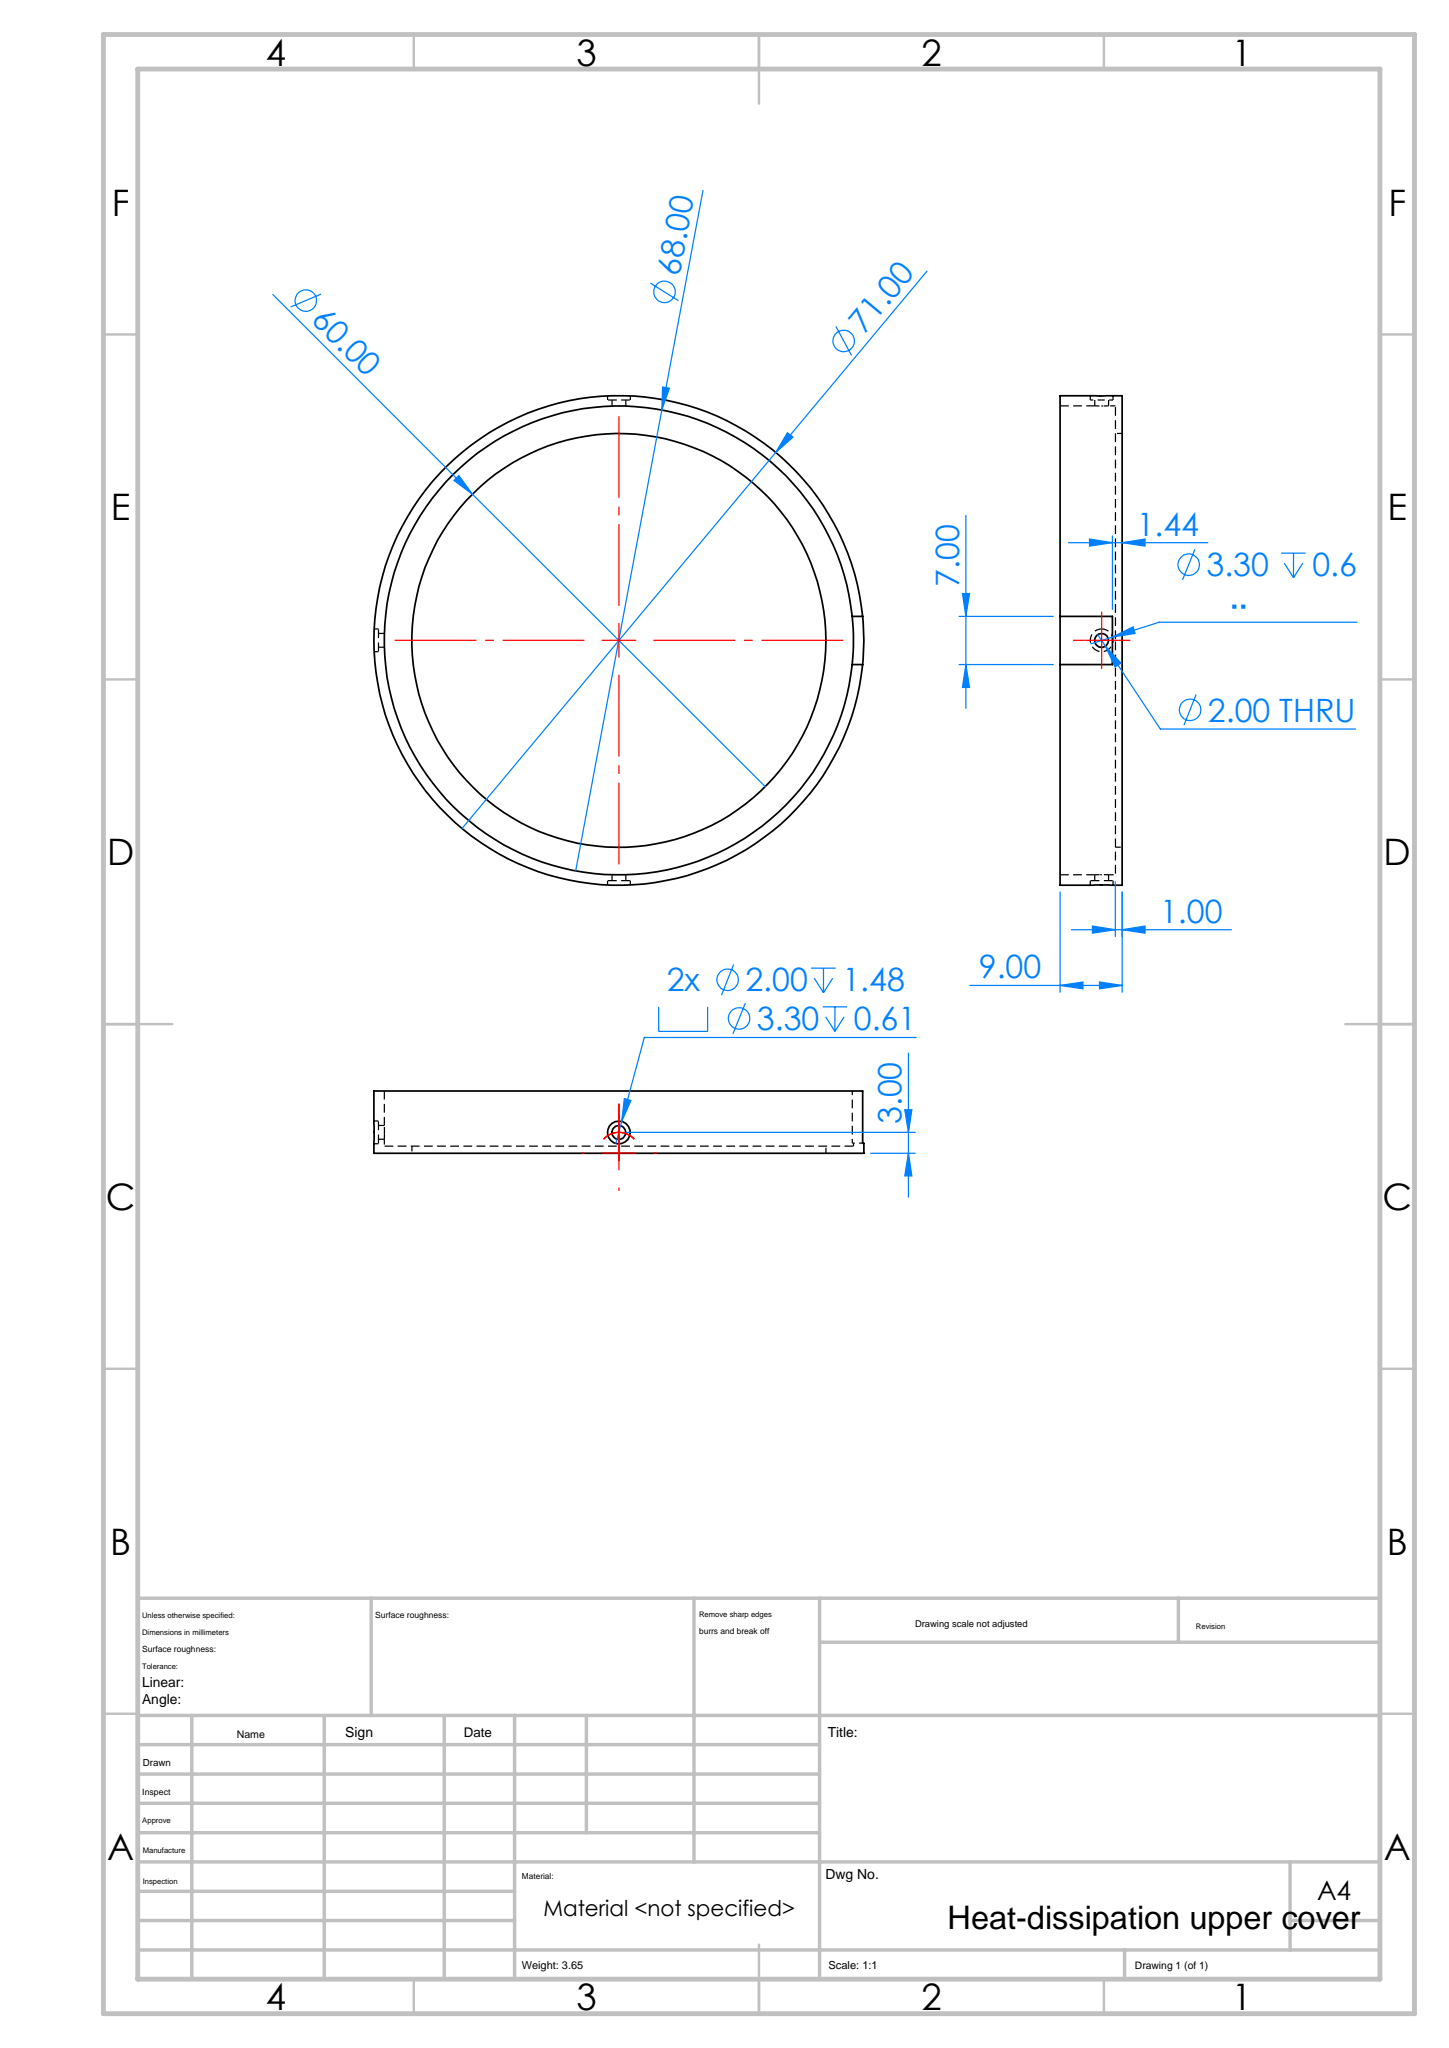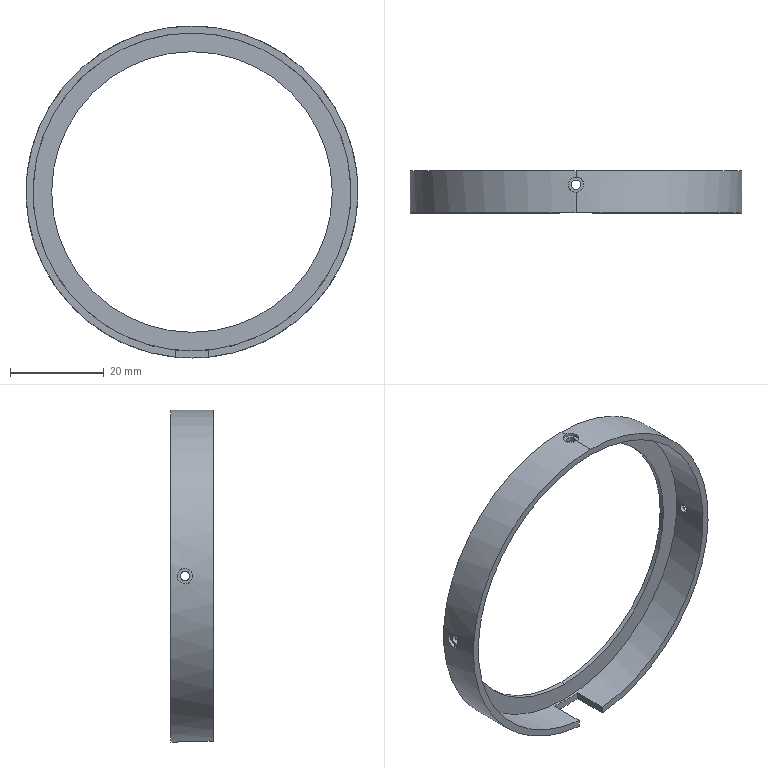Part | SolidWorks | features ICE 3, CirPattern 2, Revolution 1 | 1 solid | 27 faces | box 71 x 9 x 71 mm | volume 3648 mm3 | cylinder 18 | plane 9 | commonest cylinder face diameters 2 x6 3.3 x6 60 x2 68 x2 71 x2